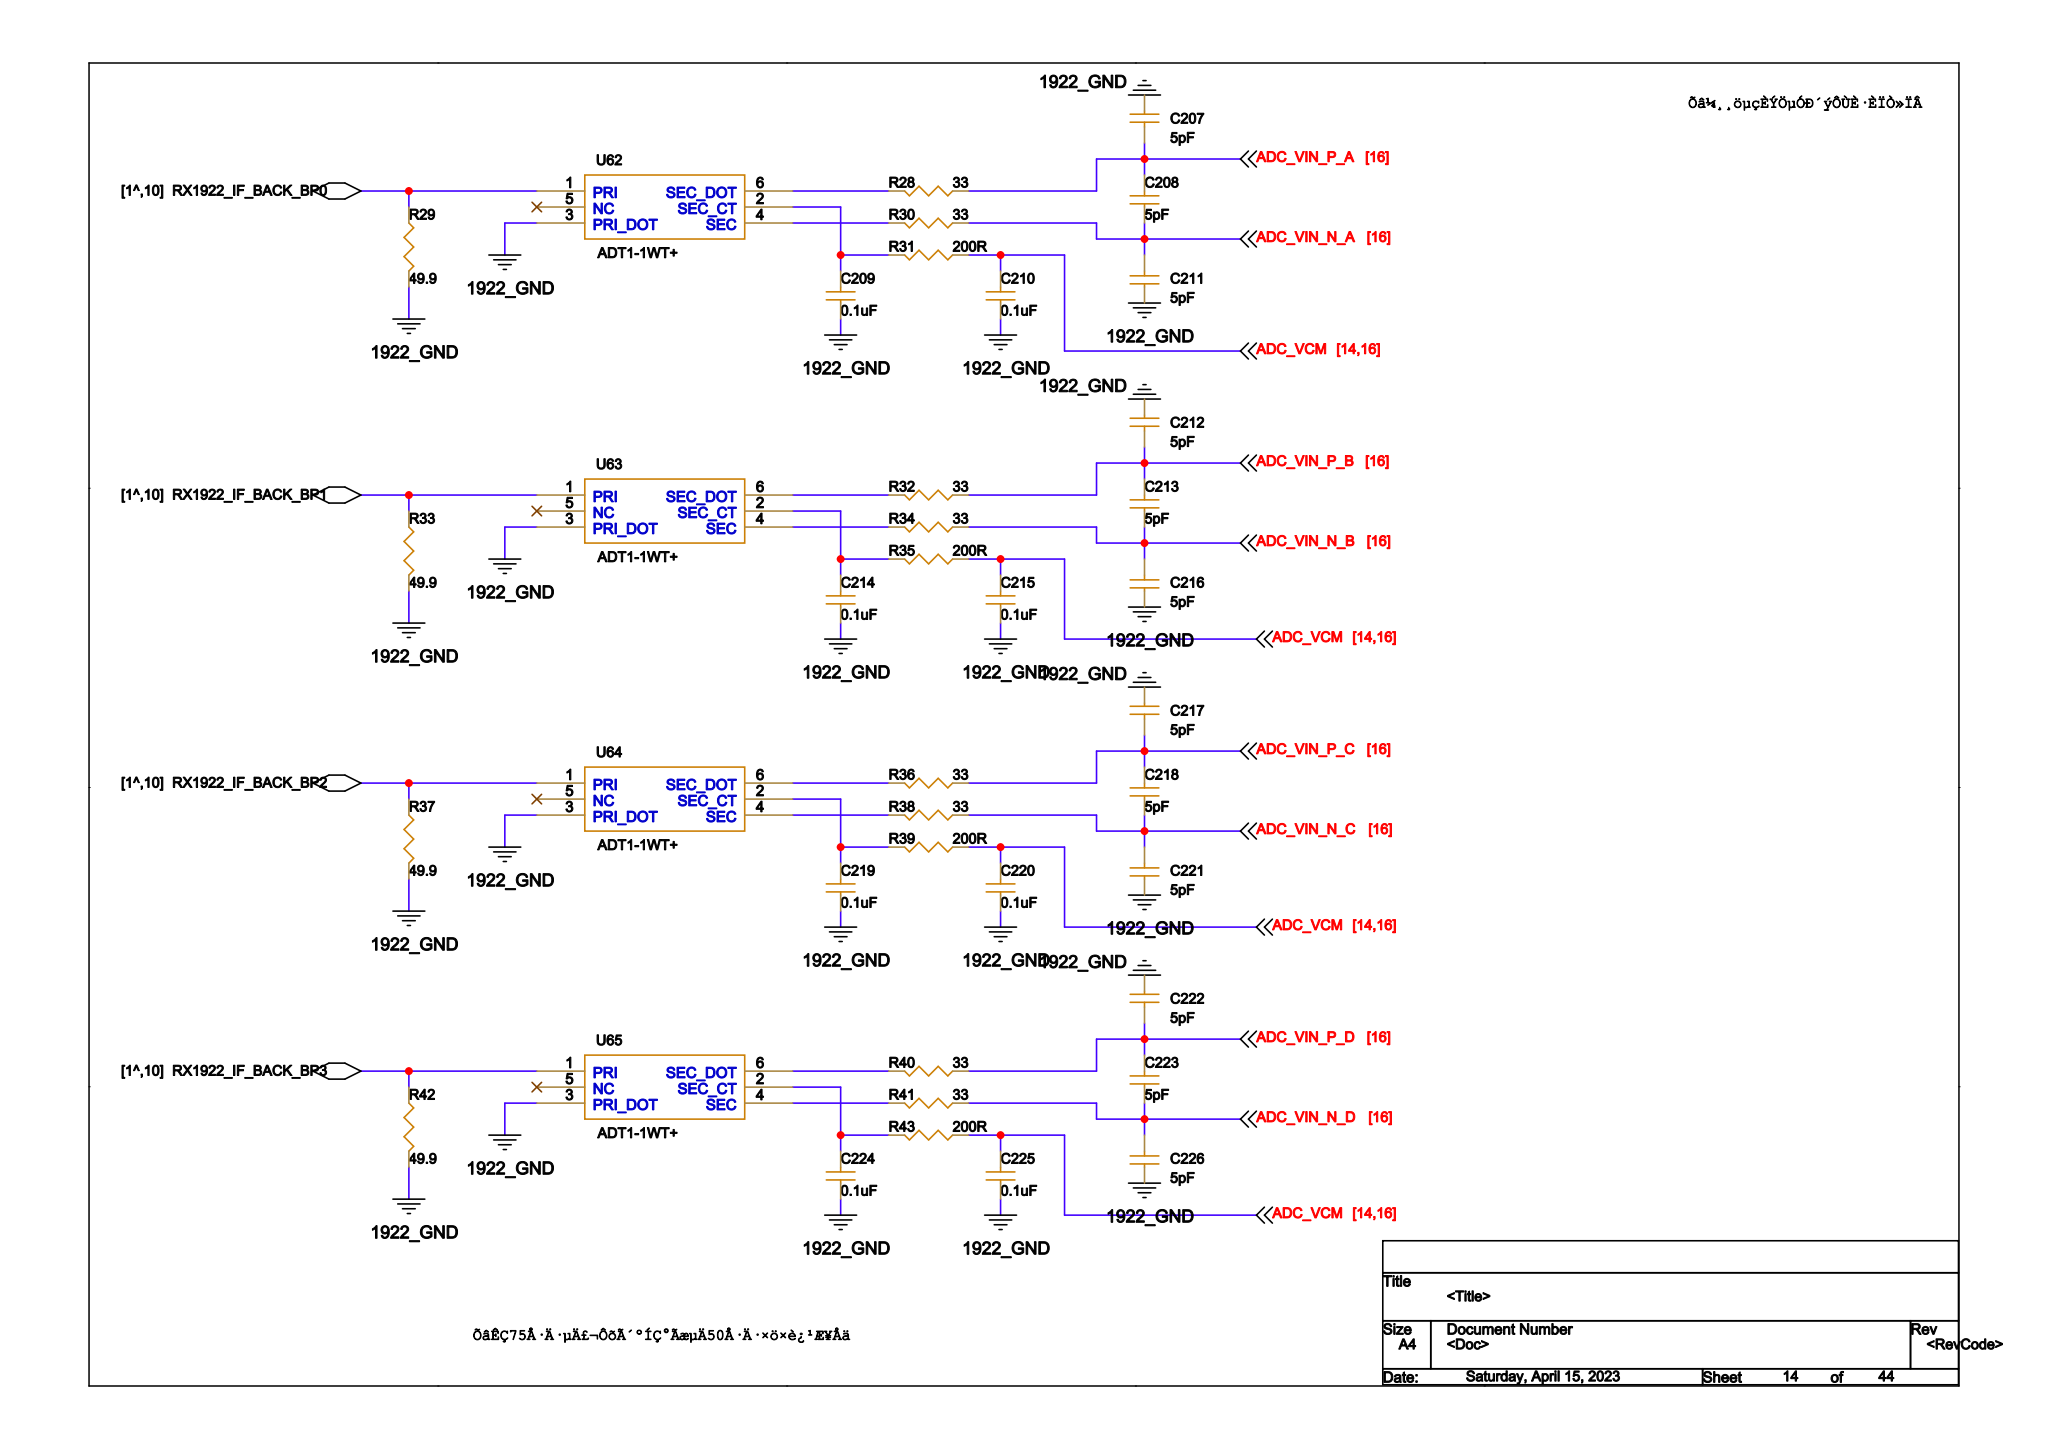Circuit board | Cadence Allegro | 1034 parts | 912 nets | one sheet of the schematic
Parts on this sheet (reference | value | footprint):
C207 | 5pF | C0402
C208 | 5pF | C0402
C209 | 0.1uF | C0402
C210 | 0.1uF | C0402
C211 | 5pF | C0402
C212 | 5pF | C0402
C213 | 5pF | C0402
C214 | 0.1uF | C0402
C215 | 0.1uF | C0402
C216 | 5pF | C0402
C217 | 5pF | C0402
C218 | 5pF | C0402
C219 | 0.1uF | C0402
C220 | 0.1uF | C0402
C221 | 5pF | C0402
C222 | 5pF | C0402
C223 | 5pF | C0402
C224 | 0.1uF | C0402
C225 | 0.1uF | C0402
C226 | 5pF | C0402
R29 | 49.9 | R0402
R31 | 200R | R0402
R32 | 33 | R0402
R33 | 49.9 | R0402
R34 | 33 | R0402
R35 | 200R | R0402
R36 | 33 | R0402
R37 | 49.9 | R0402
R38 | 33 | R0402
R39 | 200R | R0402
R40 | 33 | R0402
R41 | 33 | R0402
R42 | 49.9 | R0402
R43 | 200R | R0402
U62 | ADT1-1WT+ | ADT1_1WT_BL
U63 | ADT1-1WT+ | ADT1_1WT_BL
U64 | ADT1-1WT+ | ADT1_1WT_BL
U65 | ADT1-1WT+ | ADT1_1WT_BL
Nets of these parts (net: part-pin ...):
ADC_VCM_D3: C210-2 C215-2 C220-2 C225-2 R31-1 R35-1 R39-1 R43-1
ADC_VIN_P_A_D3: C207-2 C208-2
ADC_VIN_P_B_D3: C212-2 C213-2 R32-1
ADC_VIN_P_C_D3: C217-2 C218-2 R36-1
ADC_VIN_P_D_D3: C222-2 C223-2 R40-1
ADC_VIN_N_A_D3: C208-1 C211-2
ADC_VIN_N_B_D3: C213-1 C216-2 R34-1
ADC_VIN_N_C_D3: C218-1 C221-2 R38-1
ADC_VIN_N_D_D3: C223-1 C226-2 R41-1
1922_GND: C207-1 C209-1 C210-1 C211-1 C212-1 C214-1 C215-1 C216-1 C217-1 C219-1 C220-1 C221-1 C222-1 C224-1 C225-1 C226-1 R29-2 R33-2 R37-2 R42-2 U62-3 U63-3 U64-3 U65-3
N411903_D3: C209-2 R31-2 U62-2
N412844_D3: C214-2 R35-2 U63-2
N413577_D3: C219-2 R39-2 U64-2
N414339_D3: C224-2 R43-2 U65-2
N412892_D3: R34-2 U63-4
N413625_D3: R38-2 U64-4
N103792_D3: U62-6
N103796_D3: U62-4
N412820_D3: R32-2 U63-6
N413553_D3: R36-2 U64-6
N414315_D3: R40-2 U65-6
N414387_D3: R41-2 U65-4
N186037: R33-1 U63-1
N186039: R37-1 U64-1
N186035: R29-1 U62-1
N186041: R42-1 U65-1